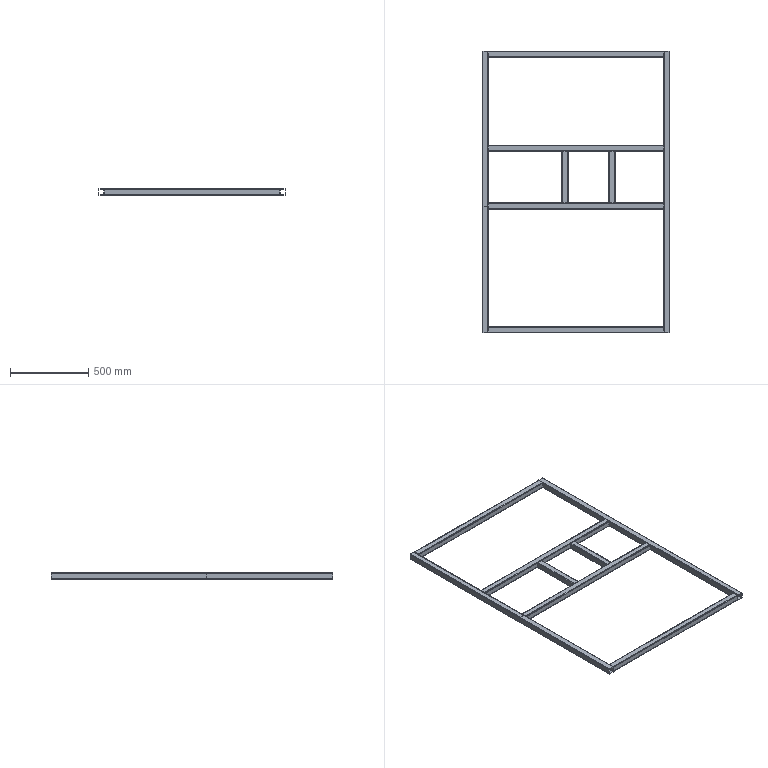Part | SolidWorks | features WeldCornerFeat 1, WeldMemberFeat 1, WeldmentFeature 1 | 9 solids | 162 faces | box 1200 x 1800 x 40 mm | volume 3242202 mm3 | plane 90 | cylinder 72 | commonest cylinder face diameters 4.6 x36 9.2 x36